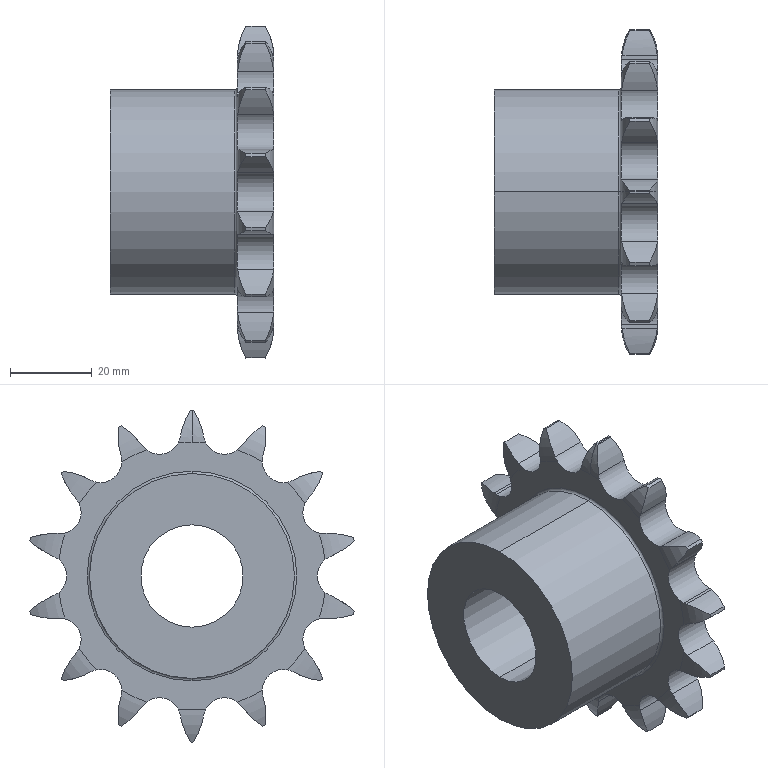Part | STEP file | short pitch roller chain wheel_s_iso_Chain wheel ISO - 14Z 10A-1 --14SB50H40L25.0N | 1 solid | 104 faces | box 40.001 x 79.165 x 81.025 mm | volume 73610 mm3 | cylinder 69 | torus 32 | plane 3 | commonest cylinder face diameters 39.014 x30 10.262 x20 81.025 x15 25 x2 50 x2